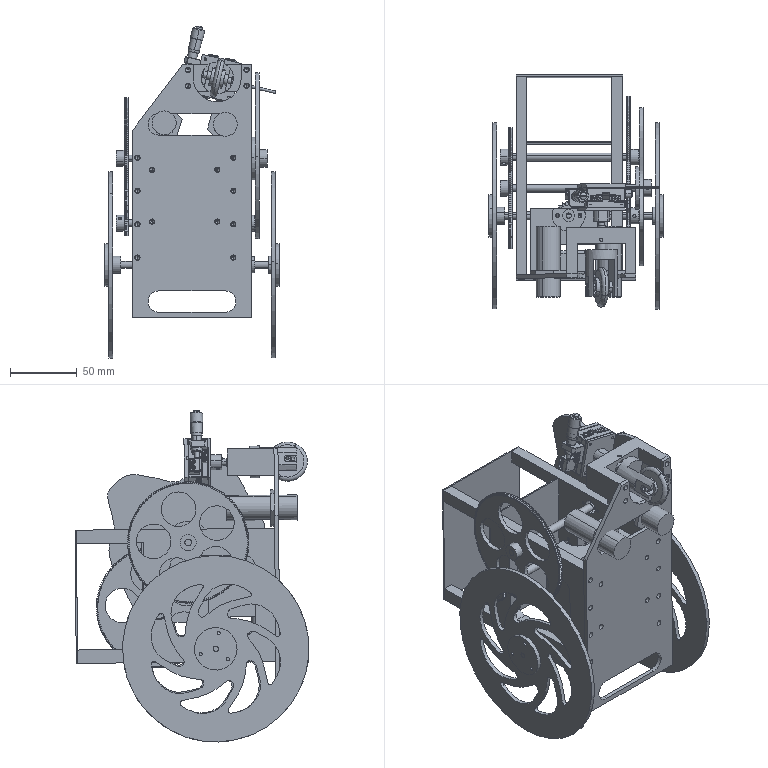Part | SolidWorks | features CompositeCurve 1, LayoutProfileFeature 1 | 34 solids | 2779 faces | box 131 x 175.611 x 249.309 mm | volume 497215 mm3 | cylinder 1125 | plane 788 | spline 506 | cone 328 | torus 20 | sphere 12 | commonest cylinder face diameters 91 x360 2.5 x73 19 x72 4 x68 2.05 x52 3.3 x48